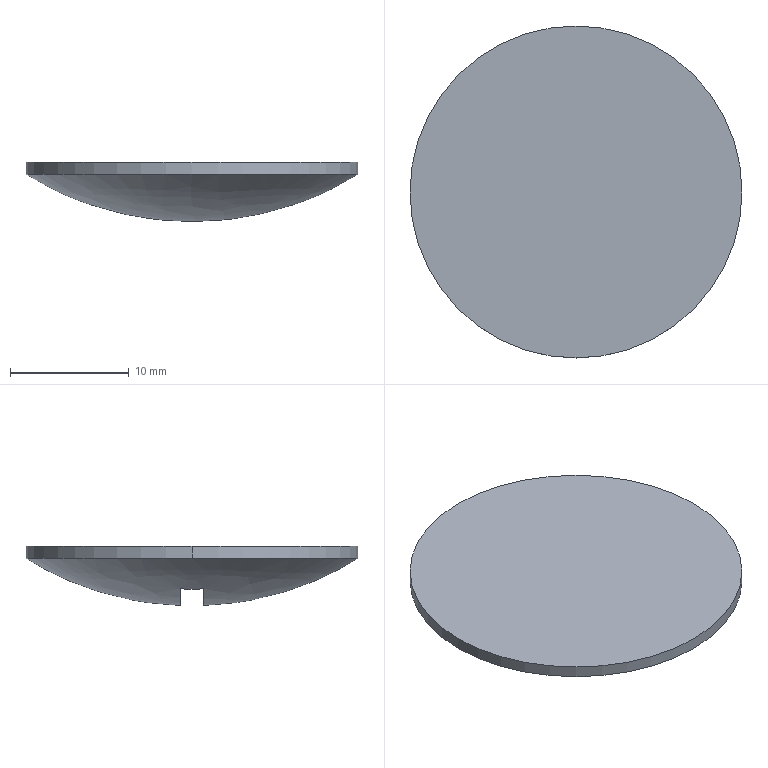Part | SolidWorks | features BaseBody 1 | 1 solid | 9 faces | box 28 x 28 x 4.981 mm | volume 1761 mm3 | plane 6 | cylinder 2 | spline 1 | commonest cylinder face diameters 28 x2
STEP:
#1=CARTESIAN_POINT('',(298.,-93.,-56.087));
#2=VERTEX_POINT('',#1);
#3=CARTESIAN_POINT('',(270.,-93.,-56.087));
#4=VERTEX_POINT('',#3);
#5=CARTESIAN_POINT('',(284.,-93.,-56.087));
#6=DIRECTION('',(0.,0.,1.));
#7=DIRECTION('',(-1.,0.,0.));
#8=AXIS2_PLACEMENT_3D('',#5,#6,#7);
#9=CIRCLE('',#8,14.);
#10=EDGE_CURVE('',#2,#4,#9,.T.);
#11=ORIENTED_EDGE('',*,*,#10,.F.);
#12=CARTESIAN_POINT('',(298.,-93.,-57.087));
#13=VERTEX_POINT('',#12);
#14=CARTESIAN_POINT('',(298.,-93.,-56.587));
#15=DIRECTION('',(0.,0.,-1.));
#16=VECTOR('',#15,1000.);
#17=LINE('',#14,#16);
#18=EDGE_CURVE('',#2,#13,#17,.T.);
#19=ORIENTED_EDGE('',*,*,#18,.T.);
#20=CARTESIAN_POINT('',(270.,-93.,-57.087));
#21=VERTEX_POINT('',#20);
#22=CARTESIAN_POINT('',(284.,-93.,-57.087));
#23=DIRECTION('',(0.,0.,1.));
#24=DIRECTION('',(-1.,0.,0.));
#25=AXIS2_PLACEMENT_3D('',#22,#23,#24);
#26=CIRCLE('',#25,14.);
#27=EDGE_CURVE('',#13,#21,#26,.T.);
#28=ORIENTED_EDGE('',*,*,#27,.T.);
#29=CARTESIAN_POINT('',(270.,-93.,-56.587));
#30=DIRECTION('',(0.,0.,-1.));
#31=VECTOR('',#30,1000.);
#32=LINE('',#29,#31);
#33=EDGE_CURVE('',#4,#21,#32,.T.);
#34=ORIENTED_EDGE('',*,*,#33,.F.);
#35=EDGE_LOOP('',(#11,#19,#28,#34));
#36=FACE_OUTER_BOUND('',#35,.T.);
#37=CARTESIAN_POINT('',(284.,-93.,-56.587));
#38=DIRECTION('',(0.,0.,-1.));
#39=DIRECTION('',(-1.,0.,0.));
#40=AXIS2_PLACEMENT_3D('',#37,#38,#39);
#41=CYLINDRICAL_SURFACE('',#40,14.);
#42=ADVANCED_FACE('',(#36),#41,.T.);
#43=CARTESIAN_POINT('',(284.,-93.,-56.087));
#44=DIRECTION('',(0.,0.,1.));
#45=DIRECTION('',(-1.,0.,0.));
#46=AXIS2_PLACEMENT_3D('',#43,#44,#45);
#47=CIRCLE('',#46,14.);
#48=EDGE_CURVE('',#4,#2,#47,.T.);
#49=ORIENTED_EDGE('',*,*,#48,.T.);
#50=ORIENTED_EDGE('',*,*,#10,.T.);
#51=EDGE_LOOP('',(#49,#50));
#52=FACE_OUTER_BOUND('',#51,.T.);
#53=CARTESIAN_POINT('',(291.,-93.,-56.087));
#54=DIRECTION('',(0.,0.,1.));
#55=DIRECTION('',(1.,0.,0.));
#56=AXIS2_PLACEMENT_3D('',#53,#54,#55);
#57=PLANE('',#56);
#58=ADVANCED_FACE('',(#52),#57,.T.);
#59=ORIENTED_EDGE('',*,*,#18,.F.);
#60=ORIENTED_EDGE('',*,*,#48,.F.);
#61=ORIENTED_EDGE('',*,*,#33,.T.);
#62=CARTESIAN_POINT('',(284.,-93.,-57.087));
#63=DIRECTION('',(0.,0.,1.));
#64=DIRECTION('',(-1.,0.,0.));
#65=AXIS2_PLACEMENT_3D('',#62,#63,#64);
#66=CIRCLE('',#65,14.);
#67=EDGE_CURVE('',#21,#13,#66,.T.);
#68=ORIENTED_EDGE('',*,*,#67,.T.);
#69=EDGE_LOOP('',(#59,#60,#61,#68));
#70=FACE_OUTER_BOUND('',#69,.T.);
#71=CARTESIAN_POINT('',(284.,-93.,-56.587));
#72=DIRECTION('',(0.,0.,-1.));
#73=DIRECTION('',(-1.,0.,0.));
#74=AXIS2_PLACEMENT_3D('',#71,#72,#73);
#75=CYLINDRICAL_SURFACE('',#74,14.);
#76=ADVANCED_FACE('',(#70),#75,.T.);
#77=CARTESIAN_POINT('',(275.5,-93.,-59.687));
#78=VERTEX_POINT('',#77);
#79=CARTESIAN_POINT('',(275.5,-92.,-59.667));
#80=VERTEX_POINT('',#79);
#81=CARTESIAN_POINT('',(275.5,-93.,-59.687));
#82=CARTESIAN_POINT('',(275.5,-92.667,-59.687));
#83=CARTESIAN_POINT('',(275.5,-92.333,-59.68));
#84=CARTESIAN_POINT('',(275.5,-92.,-59.667));
#85=B_SPLINE_CURVE_WITH_KNOTS('',3,(#81,#82,#83,#84),.UNSPECIFIED.,.F.,.F.,(4,4),(0.,1.),.UNSPECIFIED.);
#86=EDGE_CURVE('',#78,#80,#85,.T.);
#87=ORIENTED_EDGE('',*,*,#86,.F.);
#88=CARTESIAN_POINT('',(275.5,-94.,-59.667));
#89=VERTEX_POINT('',#88);
#90=CARTESIAN_POINT('',(275.5,-94.,-59.667));
#91=CARTESIAN_POINT('',(275.5,-93.667,-59.68));
#92=CARTESIAN_POINT('',(275.5,-93.333,-59.687));
#93=CARTESIAN_POINT('',(275.5,-93.,-59.687));
#94=B_SPLINE_CURVE_WITH_KNOTS('',3,(#90,#91,#92,#93),.UNSPECIFIED.,.F.,.F.,(4,4),(0.,1.),.UNSPECIFIED.);
#95=EDGE_CURVE('',#89,#78,#94,.T.);
#96=ORIENTED_EDGE('',*,*,#95,.F.);
#97=CARTESIAN_POINT('',(292.5,-94.,-59.667));
#98=VERTEX_POINT('',#97);
#99=CARTESIAN_POINT('',(275.5,-94.,-59.667));
#100=CARTESIAN_POINT('',(276.878,-94.,-60.134));
#101=CARTESIAN_POINT('',(279.674,-94.,-60.83));
#102=CARTESIAN_POINT('',(282.545,-94.,-61.068));
#103=CARTESIAN_POINT('',(285.455,-94.,-61.068));
#104=CARTESIAN_POINT('',(288.326,-94.,-60.83));
#105=CARTESIAN_POINT('',(291.122,-94.,-60.134));
#106=CARTESIAN_POINT('',(292.5,-94.,-59.667));
#107=B_SPLINE_CURVE_WITH_KNOTS('',3,(#99,#100,#101,#102,#103,#104,#105,#106),.UNSPECIFIED.,.F.,.F.,(4,1,2,1,4),(-0.008615,-0.004307,0.,0.004307,0.008615),.UNSPECIFIED.);
#108=EDGE_CURVE('',#89,#98,#107,.T.);
#109=ORIENTED_EDGE('',*,*,#108,.T.);
#110=CARTESIAN_POINT('',(292.5,-93.,-59.687));
#111=VERTEX_POINT('',#110);
#112=CARTESIAN_POINT('',(292.5,-93.,-59.687));
#113=CARTESIAN_POINT('',(292.5,-93.333,-59.687));
#114=CARTESIAN_POINT('',(292.5,-93.667,-59.68));
#115=CARTESIAN_POINT('',(292.5,-94.,-59.667));
#116=B_SPLINE_CURVE_WITH_KNOTS('',3,(#112,#113,#114,#115),.UNSPECIFIED.,.F.,.F.,(4,4),(0.,1.),.UNSPECIFIED.);
#117=EDGE_CURVE('',#111,#98,#116,.T.);
#118=ORIENTED_EDGE('',*,*,#117,.F.);
#119=CARTESIAN_POINT('',(292.5,-92.,-59.667));
#120=VERTEX_POINT('',#119);
#121=CARTESIAN_POINT('',(292.5,-92.,-59.667));
#122=CARTESIAN_POINT('',(292.5,-92.333,-59.68));
#123=CARTESIAN_POINT('',(292.5,-92.667,-59.687));
#124=CARTESIAN_POINT('',(292.5,-93.,-59.687));
#125=B_SPLINE_CURVE_WITH_KNOTS('',3,(#121,#122,#123,#124),.UNSPECIFIED.,.F.,.F.,(4,4),(0.,1.),.UNSPECIFIED.);
#126=EDGE_CURVE('',#120,#111,#125,.T.);
#127=ORIENTED_EDGE('',*,*,#126,.F.);
#128=CARTESIAN_POINT('',(292.5,-92.,-59.667));
#129=CARTESIAN_POINT('',(291.122,-92.,-60.134));
#130=CARTESIAN_POINT('',(289.725,-92.,-60.482));
#131=CARTESIAN_POINT('',(286.894,-92.,-60.949));
#132=CARTESIAN_POINT('',(285.46,-92.,-61.068));
#133=CARTESIAN_POINT('',(283.281,-92.,-61.068));
#134=CARTESIAN_POINT('',(282.555,-92.,-61.039));
#135=CARTESIAN_POINT('',(281.117,-92.,-60.921));
#136=CARTESIAN_POINT('',(280.404,-92.,-60.833));
#137=CARTESIAN_POINT('',(278.277,-92.,-60.482));
#138=CARTESIAN_POINT('',(276.878,-92.,-60.134));
#139=CARTESIAN_POINT('',(275.5,-92.,-59.667));
#140=B_SPLINE_CURVE_WITH_KNOTS('',3,(#128,#129,#130,#131,#132,#133,#134,#135,#136,#137,#138,#139),.UNSPECIFIED.,.F.,.F.,(4,2,2,2,2,4),(0.,0.004304,0.008607,0.01076,0.01291,0.01721),.UNSPECIFIED.);
#141=EDGE_CURVE('',#120,#80,#140,.T.);
#142=ORIENTED_EDGE('',*,*,#141,.T.);
#143=EDGE_LOOP('',(#87,#96,#109,#118,#127,#142));
#144=FACE_BOUND('',#143,.T.);
#145=ORIENTED_EDGE('',*,*,#67,.F.);
#146=ORIENTED_EDGE('',*,*,#27,.F.);
#147=EDGE_LOOP('',(#145,#146));
#148=FACE_OUTER_BOUND('',#147,.T.);
#149=CARTESIAN_POINT('',(271.307,-78.391,-52.689));
#150=CARTESIAN_POINT('',(269.301,-87.474,-58.613));
#151=CARTESIAN_POINT('',(269.299,-98.502,-58.618));
#152=CARTESIAN_POINT('',(271.303,-107.591,-52.701));
#153=CARTESIAN_POINT('',(280.381,-76.985,-57.918));
#154=CARTESIAN_POINT('',(278.182,-86.942,-64.412));
#155=CARTESIAN_POINT('',(278.18,-99.032,-64.417));
#156=CARTESIAN_POINT('',(280.376,-108.995,-57.931));
#157=CARTESIAN_POINT('',(290.754,-78.92,-58.463));
#158=CARTESIAN_POINT('',(288.821,-87.674,-64.172));
#159=CARTESIAN_POINT('',(288.819,-98.303,-64.176));
#160=CARTESIAN_POINT('',(290.75,-107.062,-58.474));
#161=CARTESIAN_POINT('',(299.195,-83.594,-54.155));
#162=CARTESIAN_POINT('',(297.903,-89.442,-57.969));
#163=CARTESIAN_POINT('',(297.902,-96.543,-57.972));
#164=CARTESIAN_POINT('',(299.192,-102.394,-54.162));
#165=(BOUNDED_SURFACE()B_SPLINE_SURFACE(3,3,((#149,#150,#151,#152),(#153,#154,#155,#156),(#157,#158,#159,#160),(#161,#162,#163,#164)),.UNSPECIFIED.,.F.,.F.,.F.)B_SPLINE_SURFACE_WITH_KNOTS((4,4),(4,4),(0.,1.),(0.,1.),.UNSPECIFIED.)GEOMETRIC_REPRESENTATION_ITEM()RATIONAL_B_SPLINE_SURFACE(((1.,0.8826,0.8826,1.),(0.8962,0.7909,0.7909,0.8962),(0.8962,0.7909,0.7909,0.8962),(1.,0.8826,0.8826,1.)))REPRESENTATION_ITEM('')SURFACE());
#166=ADVANCED_FACE('',(#144,#148),#165,.T.);
#167=CARTESIAN_POINT('',(292.5,-94.,-57.087));
#168=VERTEX_POINT('',#167);
#169=CARTESIAN_POINT('',(292.5,-94.,-59.587));
#170=DIRECTION('',(0.,0.,-1.));
#171=VECTOR('',#170,1000.);
#172=LINE('',#169,#171);
#173=EDGE_CURVE('',#168,#98,#172,.T.);
#174=ORIENTED_EDGE('',*,*,#173,.T.);
#175=ORIENTED_EDGE('',*,*,#108,.F.);
#176=CARTESIAN_POINT('',(275.5,-94.,-57.087));
#177=VERTEX_POINT('',#176);
#178=CARTESIAN_POINT('',(275.5,-94.,-59.587));
#179=DIRECTION('',(0.,0.,1.));
#180=VECTOR('',#179,1000.);
#181=LINE('',#178,#180);
#182=EDGE_CURVE('',#89,#177,#181,.T.);
#183=ORIENTED_EDGE('',*,*,#182,.T.);
#184=CARTESIAN_POINT('',(284.,-94.,-57.087));
#185=DIRECTION('',(1.,0.,0.));
#186=VECTOR('',#185,1000.);
#187=LINE('',#184,#186);
#188=EDGE_CURVE('',#177,#168,#187,.T.);
#189=ORIENTED_EDGE('',*,*,#188,.T.);
#190=EDGE_LOOP('',(#174,#175,#183,#189));
#191=FACE_OUTER_BOUND('',#190,.T.);
#192=CARTESIAN_POINT('',(284.,-94.,-59.587));
#193=DIRECTION('',(0.,1.,0.));
#194=DIRECTION('',(0.,0.,1.));
#195=AXIS2_PLACEMENT_3D('',#192,#193,#194);
#196=PLANE('',#195);
#197=ADVANCED_FACE('',(#191),#196,.T.);
#198=CARTESIAN_POINT('',(275.5,-92.,-57.087));
#199=VERTEX_POINT('',#198);
#200=CARTESIAN_POINT('',(275.5,-92.,-59.587));
#201=DIRECTION('',(0.,0.,-1.));
#202=VECTOR('',#201,1000.);
#203=LINE('',#200,#202);
#204=EDGE_CURVE('',#199,#80,#203,.T.);
#205=ORIENTED_EDGE('',*,*,#204,.T.);
#206=ORIENTED_EDGE('',*,*,#141,.F.);
#207=CARTESIAN_POINT('',(292.5,-92.,-57.087));
#208=VERTEX_POINT('',#207);
#209=CARTESIAN_POINT('',(292.5,-92.,-59.587));
#210=DIRECTION('',(0.,0.,1.));
#211=VECTOR('',#210,1000.);
#212=LINE('',#209,#211);
#213=EDGE_CURVE('',#120,#208,#212,.T.);
#214=ORIENTED_EDGE('',*,*,#213,.T.);
#215=CARTESIAN_POINT('',(284.,-92.,-57.087));
#216=DIRECTION('',(-1.,0.,0.));
#217=VECTOR('',#216,1000.);
#218=LINE('',#215,#217);
#219=EDGE_CURVE('',#208,#199,#218,.T.);
#220=ORIENTED_EDGE('',*,*,#219,.T.);
#221=EDGE_LOOP('',(#205,#206,#214,#220));
#222=FACE_OUTER_BOUND('',#221,.T.);
#223=CARTESIAN_POINT('',(284.,-92.,-59.587));
#224=DIRECTION('',(0.,-1.,0.));
#225=DIRECTION('',(0.,0.,-1.));
#226=AXIS2_PLACEMENT_3D('',#223,#224,#225);
#227=PLANE('',#226);
#228=ADVANCED_FACE('',(#222),#227,.T.);
#229=ORIENTED_EDGE('',*,*,#126,.T.);
#230=ORIENTED_EDGE('',*,*,#117,.T.);
#231=ORIENTED_EDGE('',*,*,#173,.F.);
#232=CARTESIAN_POINT('',(292.5,-93.,-57.087));
#233=DIRECTION('',(0.,1.,0.));
#234=VECTOR('',#233,1000.);
#235=LINE('',#232,#234);
#236=EDGE_CURVE('',#168,#208,#235,.T.);
#237=ORIENTED_EDGE('',*,*,#236,.T.);
#238=ORIENTED_EDGE('',*,*,#213,.F.);
#239=EDGE_LOOP('',(#229,#230,#231,#237,#238));
#240=FACE_OUTER_BOUND('',#239,.T.);
#241=CARTESIAN_POINT('',(292.5,-93.,-59.587));
#242=DIRECTION('',(-1.,0.,0.));
#243=DIRECTION('',(0.,0.,1.));
#244=AXIS2_PLACEMENT_3D('',#241,#242,#243);
#245=PLANE('',#244);
#246=ADVANCED_FACE('',(#240),#245,.T.);
#247=ORIENTED_EDGE('',*,*,#219,.F.);
#248=ORIENTED_EDGE('',*,*,#236,.F.);
#249=ORIENTED_EDGE('',*,*,#188,.F.);
#250=CARTESIAN_POINT('',(275.5,-93.,-57.087));
#251=DIRECTION('',(0.,1.,0.));
#252=VECTOR('',#251,1000.);
#253=LINE('',#250,#252);
#254=EDGE_CURVE('',#177,#199,#253,.T.);
#255=ORIENTED_EDGE('',*,*,#254,.T.);
#256=EDGE_LOOP('',(#247,#248,#249,#255));
#257=FACE_OUTER_BOUND('',#256,.T.);
#258=CARTESIAN_POINT('',(284.,-93.,-57.087));
#259=DIRECTION('',(0.,0.,-1.));
#260=DIRECTION('',(-1.,0.,0.));
#261=AXIS2_PLACEMENT_3D('',#258,#259,#260);
#262=PLANE('',#261);
#263=ADVANCED_FACE('',(#257),#262,.T.);
#264=ORIENTED_EDGE('',*,*,#95,.T.);
#265=ORIENTED_EDGE('',*,*,#86,.T.);
#266=ORIENTED_EDGE('',*,*,#204,.F.);
#267=ORIENTED_EDGE('',*,*,#254,.F.);
#268=ORIENTED_EDGE('',*,*,#182,.F.);
#269=EDGE_LOOP('',(#264,#265,#266,#267,#268));
#270=FACE_OUTER_BOUND('',#269,.T.);
#271=CARTESIAN_POINT('',(275.5,-93.,-59.587));
#272=DIRECTION('',(1.,0.,0.));
#273=DIRECTION('',(0.,0.,-1.));
#274=AXIS2_PLACEMENT_3D('',#271,#272,#273);
#275=PLANE('',#274);
#276=ADVANCED_FACE('',(#270),#275,.T.);
#277=CLOSED_SHELL('',(#42,#58,#76,#166,#197,#228,#246,#263,#276));
#278=MANIFOLD_SOLID_BREP('',#277);
#279=CARTESIAN_POINT('',(0.,0.,0.));
#280=DIRECTION('',(0.,0.,1.));
#281=DIRECTION('',(1.,0.,0.));
#282=AXIS2_PLACEMENT_3D('',#279,#280,#281);
#283=(LENGTH_UNIT()NAMED_UNIT(*)SI_UNIT(.MILLI.,.METRE.));
#284=UNCERTAINTY_MEASURE_WITH_UNIT(LENGTH_MEASURE(0.00001),#283,'','');
#285=(NAMED_UNIT(*)PLANE_ANGLE_UNIT()SI_UNIT($,.RADIAN.));
#286=(NAMED_UNIT(*)SI_UNIT($,.STERADIAN.)SOLID_ANGLE_UNIT());
#287=(GEOMETRIC_REPRESENTATION_CONTEXT(3)GLOBAL_UNCERTAINTY_ASSIGNED_CONTEXT((#284))GLOBAL_UNIT_ASSIGNED_CONTEXT((#283,#285,#286))REPRESENTATION_CONTEXT('',''));
#288=ADVANCED_BREP_SHAPE_REPRESENTATION('',(#278,#282),#287);